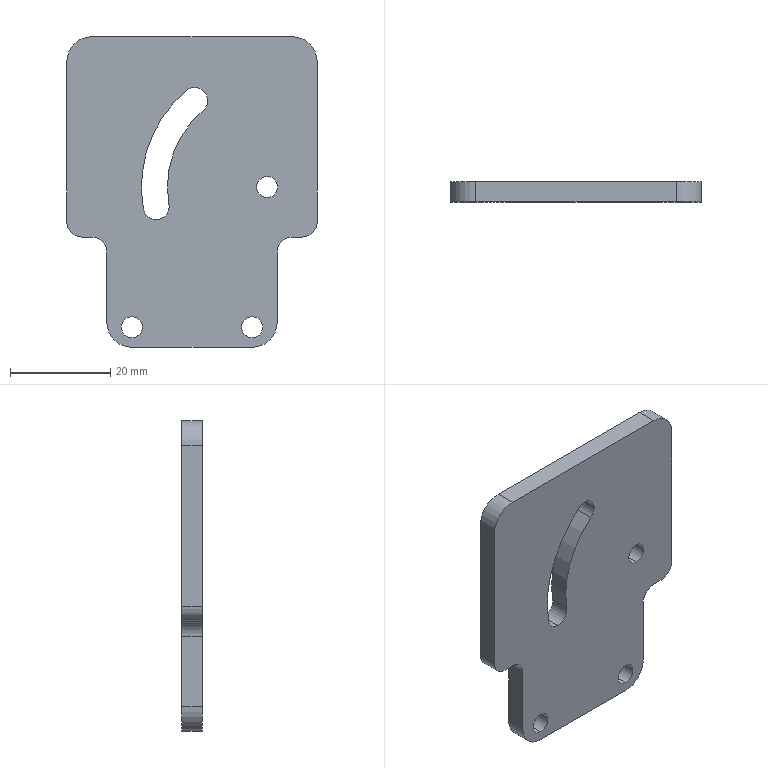Part | SolidWorks | features BaseBody 1 | 1 solid | 29 faces | box 50 x 4 x 62 mm | volume 10165 mm3 | cylinder 19 | plane 10 | commonest cylinder face diameters 4.2 x6 6 x4 10 x4 5.2 x3 39.8 x1 50.2 x1
STEP:
#1=CARTESIAN_POINT('',(-27.,0.,-25.9));
#2=VERTEX_POINT('',#1);
#3=CARTESIAN_POINT('',(-27.,0.,-30.1));
#4=VERTEX_POINT('',#3);
#5=CARTESIAN_POINT('',(-27.,0.,-28.));
#6=DIRECTION('',(0.,-1.,0.));
#7=DIRECTION('',(0.,0.,1.));
#8=AXIS2_PLACEMENT_3D('',#5,#6,#7);
#9=CIRCLE('',#8,2.1);
#10=EDGE_CURVE('',#2,#4,#9,.T.);
#11=ORIENTED_EDGE('',*,*,#10,.T.);
#12=CARTESIAN_POINT('',(-27.,4.,-30.1));
#13=VERTEX_POINT('',#12);
#14=CARTESIAN_POINT('',(-27.,0.,-30.1));
#15=DIRECTION('',(0.,1.,0.));
#16=VECTOR('',#15,1000.);
#17=LINE('',#14,#16);
#18=EDGE_CURVE('',#4,#13,#17,.T.);
#19=ORIENTED_EDGE('',*,*,#18,.T.);
#20=CARTESIAN_POINT('',(-27.,4.,-25.9));
#21=VERTEX_POINT('',#20);
#22=CARTESIAN_POINT('',(-27.,4.,-28.));
#23=DIRECTION('',(0.,-1.,0.));
#24=DIRECTION('',(0.,0.,1.));
#25=AXIS2_PLACEMENT_3D('',#22,#23,#24);
#26=CIRCLE('',#25,2.1);
#27=EDGE_CURVE('',#21,#13,#26,.T.);
#28=ORIENTED_EDGE('',*,*,#27,.F.);
#29=CARTESIAN_POINT('',(-27.,0.,-25.9));
#30=DIRECTION('',(0.,1.,0.));
#31=VECTOR('',#30,1000.);
#32=LINE('',#29,#31);
#33=EDGE_CURVE('',#2,#21,#32,.T.);
#34=ORIENTED_EDGE('',*,*,#33,.F.);
#35=EDGE_LOOP('',(#11,#19,#28,#34));
#36=FACE_OUTER_BOUND('',#35,.T.);
#37=CARTESIAN_POINT('',(-27.,0.,-28.));
#38=DIRECTION('',(0.,1.,0.));
#39=DIRECTION('',(0.,0.,1.));
#40=AXIS2_PLACEMENT_3D('',#37,#38,#39);
#41=CYLINDRICAL_SURFACE('',#40,2.1);
#42=ADVANCED_FACE('',(#36),#41,.F.);
#43=CARTESIAN_POINT('',(-3.,0.,-25.9));
#44=VERTEX_POINT('',#43);
#45=CARTESIAN_POINT('',(-3.,0.,-30.1));
#46=VERTEX_POINT('',#45);
#47=CARTESIAN_POINT('',(-3.,0.,-28.));
#48=DIRECTION('',(0.,-1.,0.));
#49=DIRECTION('',(0.,0.,1.));
#50=AXIS2_PLACEMENT_3D('',#47,#48,#49);
#51=CIRCLE('',#50,2.1);
#52=EDGE_CURVE('',#44,#46,#51,.T.);
#53=ORIENTED_EDGE('',*,*,#52,.T.);
#54=CARTESIAN_POINT('',(-3.,4.,-30.1));
#55=VERTEX_POINT('',#54);
#56=CARTESIAN_POINT('',(-3.,0.,-30.1));
#57=DIRECTION('',(0.,1.,0.));
#58=VECTOR('',#57,1000.);
#59=LINE('',#56,#58);
#60=EDGE_CURVE('',#46,#55,#59,.T.);
#61=ORIENTED_EDGE('',*,*,#60,.T.);
#62=CARTESIAN_POINT('',(-3.,4.,-25.9));
#63=VERTEX_POINT('',#62);
#64=CARTESIAN_POINT('',(-3.,4.,-28.));
#65=DIRECTION('',(0.,-1.,0.));
#66=DIRECTION('',(0.,0.,1.));
#67=AXIS2_PLACEMENT_3D('',#64,#65,#66);
#68=CIRCLE('',#67,2.1);
#69=EDGE_CURVE('',#63,#55,#68,.T.);
#70=ORIENTED_EDGE('',*,*,#69,.F.);
#71=CARTESIAN_POINT('',(-3.,0.,-25.9));
#72=DIRECTION('',(0.,1.,0.));
#73=VECTOR('',#72,1000.);
#74=LINE('',#71,#73);
#75=EDGE_CURVE('',#44,#63,#74,.T.);
#76=ORIENTED_EDGE('',*,*,#75,.F.);
#77=EDGE_LOOP('',(#53,#61,#70,#76));
#78=FACE_OUTER_BOUND('',#77,.T.);
#79=CARTESIAN_POINT('',(-3.,0.,-28.));
#80=DIRECTION('',(0.,1.,0.));
#81=DIRECTION('',(0.,0.,1.));
#82=AXIS2_PLACEMENT_3D('',#79,#80,#81);
#83=CYLINDRICAL_SURFACE('',#82,2.1);
#84=ADVANCED_FACE('',(#78),#83,.F.);
#85=CARTESIAN_POINT('',(-22.158,4.,-6.507));
#86=VERTEX_POINT('',#85);
#87=CARTESIAN_POINT('',(-19.598,4.,-3.456));
#88=VERTEX_POINT('',#87);
#89=CARTESIAN_POINT('',(-22.158,4.,-3.907));
#90=DIRECTION('',(0.,-1.,0.));
#91=DIRECTION('',(0.,0.,-1.));
#92=AXIS2_PLACEMENT_3D('',#89,#90,#91);
#93=CIRCLE('',#92,2.6);
#94=EDGE_CURVE('',#86,#88,#93,.T.);
#95=ORIENTED_EDGE('',*,*,#94,.F.);
#96=CARTESIAN_POINT('',(-22.158,0.,-6.507));
#97=VERTEX_POINT('',#96);
#98=CARTESIAN_POINT('',(-22.158,4.,-6.507));
#99=DIRECTION('',(0.,-1.,0.));
#100=VECTOR('',#99,1000.);
#101=LINE('',#98,#100);
#102=EDGE_CURVE('',#86,#97,#101,.T.);
#103=ORIENTED_EDGE('',*,*,#102,.T.);
#104=CARTESIAN_POINT('',(-19.598,0.,-3.456));
#105=VERTEX_POINT('',#104);
#106=CARTESIAN_POINT('',(-22.158,0.,-3.907));
#107=DIRECTION('',(0.,-1.,0.));
#108=DIRECTION('',(0.,0.,-1.));
#109=AXIS2_PLACEMENT_3D('',#106,#107,#108);
#110=CIRCLE('',#109,2.6);
#111=EDGE_CURVE('',#97,#105,#110,.T.);
#112=ORIENTED_EDGE('',*,*,#111,.T.);
#113=CARTESIAN_POINT('',(-19.598,4.,-3.456));
#114=DIRECTION('',(0.,-1.,0.));
#115=VECTOR('',#114,1000.);
#116=LINE('',#113,#115);
#117=EDGE_CURVE('',#88,#105,#116,.T.);
#118=ORIENTED_EDGE('',*,*,#117,.F.);
#119=EDGE_LOOP('',(#95,#103,#112,#118));
#120=FACE_OUTER_BOUND('',#119,.T.);
#121=CARTESIAN_POINT('',(-22.158,4.,-3.907));
#122=DIRECTION('',(0.,-1.,0.));
#123=DIRECTION('',(0.,0.,-1.));
#124=AXIS2_PLACEMENT_3D('',#121,#122,#123);
#125=CYLINDRICAL_SURFACE('',#124,2.6);
#126=ADVANCED_FACE('',(#120),#125,.F.);
#127=CARTESIAN_POINT('',(0.,4.,2.1));
#128=VERTEX_POINT('',#127);
#129=CARTESIAN_POINT('',(0.,4.,-2.1));
#130=VERTEX_POINT('',#129);
#131=CARTESIAN_POINT('',(0.,4.,0.));
#132=DIRECTION('',(0.,-1.,0.));
#133=DIRECTION('',(0.,0.,-1.));
#134=AXIS2_PLACEMENT_3D('',#131,#132,#133);
#135=CIRCLE('',#134,2.1);
#136=EDGE_CURVE('',#128,#130,#135,.T.);
#137=ORIENTED_EDGE('',*,*,#136,.F.);
#138=CARTESIAN_POINT('',(0.,0.,2.1));
#139=VERTEX_POINT('',#138);
#140=CARTESIAN_POINT('',(0.,4.,2.1));
#141=DIRECTION('',(0.,-1.,0.));
#142=VECTOR('',#141,1000.);
#143=LINE('',#140,#142);
#144=EDGE_CURVE('',#128,#139,#143,.T.);
#145=ORIENTED_EDGE('',*,*,#144,.T.);
#146=CARTESIAN_POINT('',(0.,0.,-2.1));
#147=VERTEX_POINT('',#146);
#148=CARTESIAN_POINT('',(0.,0.,0.));
#149=DIRECTION('',(0.,-1.,0.));
#150=DIRECTION('',(0.,0.,-1.));
#151=AXIS2_PLACEMENT_3D('',#148,#149,#150);
#152=CIRCLE('',#151,2.1);
#153=EDGE_CURVE('',#139,#147,#152,.T.);
#154=ORIENTED_EDGE('',*,*,#153,.T.);
#155=CARTESIAN_POINT('',(0.,4.,-2.1));
#156=DIRECTION('',(0.,-1.,0.));
#157=VECTOR('',#156,1000.);
#158=LINE('',#155,#157);
#159=EDGE_CURVE('',#130,#147,#158,.T.);
#160=ORIENTED_EDGE('',*,*,#159,.F.);
#161=EDGE_LOOP('',(#137,#145,#154,#160));
#162=FACE_OUTER_BOUND('',#161,.T.);
#163=CARTESIAN_POINT('',(0.,4.,0.));
#164=DIRECTION('',(0.,-1.,0.));
#165=DIRECTION('',(0.,0.,-1.));
#166=AXIS2_PLACEMENT_3D('',#163,#164,#165);
#167=CYLINDRICAL_SURFACE('',#166,2.1);
#168=ADVANCED_FACE('',(#162),#167,.F.);
#169=ORIENTED_EDGE('',*,*,#10,.F.);
#170=CARTESIAN_POINT('',(-27.,0.,-28.));
#171=DIRECTION('',(0.,-1.,0.));
#172=DIRECTION('',(0.,0.,1.));
#173=AXIS2_PLACEMENT_3D('',#170,#171,#172);
#174=CIRCLE('',#173,2.1);
#175=EDGE_CURVE('',#4,#2,#174,.T.);
#176=ORIENTED_EDGE('',*,*,#175,.F.);
#177=EDGE_LOOP('',(#169,#176));
#178=FACE_BOUND('',#177,.T.);
#179=ORIENTED_EDGE('',*,*,#52,.F.);
#180=CARTESIAN_POINT('',(-3.,0.,-28.));
#181=DIRECTION('',(0.,-1.,0.));
#182=DIRECTION('',(0.,0.,1.));
#183=AXIS2_PLACEMENT_3D('',#180,#181,#182);
#184=CIRCLE('',#183,2.1);
#185=EDGE_CURVE('',#46,#44,#184,.T.);
#186=ORIENTED_EDGE('',*,*,#185,.F.);
#187=EDGE_LOOP('',(#179,#186));
#188=FACE_BOUND('',#187,.T.);
#189=CARTESIAN_POINT('',(-24.719,0.,-4.359));
#190=VERTEX_POINT('',#189);
#191=CARTESIAN_POINT('',(-22.158,0.,-3.907));
#192=DIRECTION('',(0.,-1.,0.));
#193=DIRECTION('',(0.,0.,-1.));
#194=AXIS2_PLACEMENT_3D('',#191,#192,#193);
#195=CIRCLE('',#194,2.6);
#196=EDGE_CURVE('',#190,#97,#195,.T.);
#197=ORIENTED_EDGE('',*,*,#196,.F.);
#198=CARTESIAN_POINT('',(-16.134,0.,19.228));
#199=VERTEX_POINT('',#198);
#200=CARTESIAN_POINT('',(0.,0.,0.));
#201=DIRECTION('',(0.,-1.,0.));
#202=DIRECTION('',(0.,0.,-1.));
#203=AXIS2_PLACEMENT_3D('',#200,#201,#202);
#204=CIRCLE('',#203,25.1);
#205=EDGE_CURVE('',#199,#190,#204,.T.);
#206=ORIENTED_EDGE('',*,*,#205,.F.);
#207=CARTESIAN_POINT('',(-12.791,0.,15.244));
#208=VERTEX_POINT('',#207);
#209=CARTESIAN_POINT('',(-14.463,0.,17.236));
#210=DIRECTION('',(0.,-1.,0.));
#211=DIRECTION('',(0.,0.,-1.));
#212=AXIS2_PLACEMENT_3D('',#209,#210,#211);
#213=CIRCLE('',#212,2.6);
#214=EDGE_CURVE('',#208,#199,#213,.T.);
#215=ORIENTED_EDGE('',*,*,#214,.F.);
#216=CARTESIAN_POINT('',(0.,0.,0.));
#217=DIRECTION('',(0.,1.,0.));
#218=DIRECTION('',(0.,0.,-1.));
#219=AXIS2_PLACEMENT_3D('',#216,#217,#218);
#220=CIRCLE('',#219,19.9);
#221=EDGE_CURVE('',#105,#208,#220,.T.);
#222=ORIENTED_EDGE('',*,*,#221,.F.);
#223=ORIENTED_EDGE('',*,*,#111,.F.);
#224=EDGE_LOOP('',(#197,#206,#215,#222,#223));
#225=FACE_BOUND('',#224,.T.);
#226=CARTESIAN_POINT('',(2.,0.,-27.));
#227=VERTEX_POINT('',#226);
#228=CARTESIAN_POINT('',(-3.,0.,-32.));
#229=VERTEX_POINT('',#228);
#230=CARTESIAN_POINT('',(-3.,0.,-27.));
#231=DIRECTION('',(0.,1.,0.));
#232=DIRECTION('',(0.,0.,1.));
#233=AXIS2_PLACEMENT_3D('',#230,#231,#232);
#234=CIRCLE('',#233,5.);
#235=EDGE_CURVE('',#227,#229,#234,.T.);
#236=ORIENTED_EDGE('',*,*,#235,.F.);
#237=CARTESIAN_POINT('',(2.,0.,-13.));
#238=VERTEX_POINT('',#237);
#239=CARTESIAN_POINT('',(2.,0.,0.));
#240=DIRECTION('',(0.,0.,-1.));
#241=VECTOR('',#240,1000.);
#242=LINE('',#239,#241);
#243=EDGE_CURVE('',#238,#227,#242,.T.);
#244=ORIENTED_EDGE('',*,*,#243,.F.);
#245=CARTESIAN_POINT('',(5.,0.,-10.));
#246=VERTEX_POINT('',#245);
#247=CARTESIAN_POINT('',(5.,0.,-13.));
#248=DIRECTION('',(0.,-1.,0.));
#249=DIRECTION('',(0.,0.,-1.));
#250=AXIS2_PLACEMENT_3D('',#247,#248,#249);
#251=CIRCLE('',#250,3.);
#252=EDGE_CURVE('',#246,#238,#251,.T.);
#253=ORIENTED_EDGE('',*,*,#252,.F.);
#254=CARTESIAN_POINT('',(7.,0.,-10.));
#255=VERTEX_POINT('',#254);
#256=CARTESIAN_POINT('',(0.,0.,-10.));
#257=DIRECTION('',(-1.,0.,0.));
#258=VECTOR('',#257,1000.);
#259=LINE('',#256,#258);
#260=EDGE_CURVE('',#255,#246,#259,.T.);
#261=ORIENTED_EDGE('',*,*,#260,.F.);
#262=CARTESIAN_POINT('',(10.,0.,-7.));
#263=VERTEX_POINT('',#262);
#264=CARTESIAN_POINT('',(7.,0.,-7.));
#265=DIRECTION('',(0.,1.,0.));
#266=DIRECTION('',(0.,0.,-1.));
#267=AXIS2_PLACEMENT_3D('',#264,#265,#266);
#268=CIRCLE('',#267,3.);
#269=EDGE_CURVE('',#263,#255,#268,.T.);
#270=ORIENTED_EDGE('',*,*,#269,.F.);
#271=CARTESIAN_POINT('',(10.,0.,25.));
#272=VERTEX_POINT('',#271);
#273=CARTESIAN_POINT('',(10.,0.,0.));
#274=DIRECTION('',(0.,0.,-1.));
#275=VECTOR('',#274,1000.);
#276=LINE('',#273,#275);
#277=EDGE_CURVE('',#272,#263,#276,.T.);
#278=ORIENTED_EDGE('',*,*,#277,.F.);
#279=CARTESIAN_POINT('',(5.,0.,30.));
#280=VERTEX_POINT('',#279);
#281=CARTESIAN_POINT('',(5.,0.,25.));
#282=DIRECTION('',(0.,1.,0.));
#283=DIRECTION('',(0.,0.,-1.));
#284=AXIS2_PLACEMENT_3D('',#281,#282,#283);
#285=CIRCLE('',#284,5.);
#286=EDGE_CURVE('',#280,#272,#285,.T.);
#287=ORIENTED_EDGE('',*,*,#286,.F.);
#288=CARTESIAN_POINT('',(-35.,0.,30.));
#289=VERTEX_POINT('',#288);
#290=CARTESIAN_POINT('',(0.,0.,30.));
#291=DIRECTION('',(1.,0.,0.));
#292=VECTOR('',#291,1000.);
#293=LINE('',#290,#292);
#294=EDGE_CURVE('',#289,#280,#293,.T.);
#295=ORIENTED_EDGE('',*,*,#294,.F.);
#296=CARTESIAN_POINT('',(-40.,0.,25.));
#297=VERTEX_POINT('',#296);
#298=CARTESIAN_POINT('',(-35.,0.,25.));
#299=DIRECTION('',(0.,1.,0.));
#300=DIRECTION('',(0.,0.,-1.));
#301=AXIS2_PLACEMENT_3D('',#298,#299,#300);
#302=CIRCLE('',#301,5.);
#303=EDGE_CURVE('',#297,#289,#302,.T.);
#304=ORIENTED_EDGE('',*,*,#303,.F.);
#305=CARTESIAN_POINT('',(-40.,0.,-7.));
#306=VERTEX_POINT('',#305);
#307=CARTESIAN_POINT('',(-40.,0.,0.));
#308=DIRECTION('',(0.,0.,1.));
#309=VECTOR('',#308,1000.);
#310=LINE('',#307,#309);
#311=EDGE_CURVE('',#306,#297,#310,.T.);
#312=ORIENTED_EDGE('',*,*,#311,.F.);
#313=CARTESIAN_POINT('',(-37.,0.,-10.));
#314=VERTEX_POINT('',#313);
#315=CARTESIAN_POINT('',(-37.,0.,-7.));
#316=DIRECTION('',(0.,1.,0.));
#317=DIRECTION('',(0.,0.,-1.));
#318=AXIS2_PLACEMENT_3D('',#315,#316,#317);
#319=CIRCLE('',#318,3.);
#320=EDGE_CURVE('',#314,#306,#319,.T.);
#321=ORIENTED_EDGE('',*,*,#320,.F.);
#322=CARTESIAN_POINT('',(-35.,0.,-10.));
#323=VERTEX_POINT('',#322);
#324=CARTESIAN_POINT('',(0.,0.,-10.));
#325=DIRECTION('',(-1.,0.,0.));
#326=VECTOR('',#325,1000.);
#327=LINE('',#324,#326);
#328=EDGE_CURVE('',#323,#314,#327,.T.);
#329=ORIENTED_EDGE('',*,*,#328,.F.);
#330=CARTESIAN_POINT('',(-32.,0.,-13.));
#331=VERTEX_POINT('',#330);
#332=CARTESIAN_POINT('',(-35.,0.,-13.));
#333=DIRECTION('',(0.,-1.,0.));
#334=DIRECTION('',(0.,0.,1.));
#335=AXIS2_PLACEMENT_3D('',#332,#333,#334);
#336=CIRCLE('',#335,3.);
#337=EDGE_CURVE('',#331,#323,#336,.T.);
#338=ORIENTED_EDGE('',*,*,#337,.F.);
#339=CARTESIAN_POINT('',(-32.,0.,-27.));
#340=VERTEX_POINT('',#339);
#341=CARTESIAN_POINT('',(-32.,0.,0.));
#342=DIRECTION('',(0.,0.,1.));
#343=VECTOR('',#342,1000.);
#344=LINE('',#341,#343);
#345=EDGE_CURVE('',#340,#331,#344,.T.);
#346=ORIENTED_EDGE('',*,*,#345,.F.);
#347=CARTESIAN_POINT('',(-27.,0.,-32.));
#348=VERTEX_POINT('',#347);
#349=CARTESIAN_POINT('',(-27.,0.,-27.));
#350=DIRECTION('',(0.,1.,0.));
#351=DIRECTION('',(0.,0.,-1.));
#352=AXIS2_PLACEMENT_3D('',#349,#350,#351);
#353=CIRCLE('',#352,5.);
#354=EDGE_CURVE('',#348,#340,#353,.T.);
#355=ORIENTED_EDGE('',*,*,#354,.F.);
#356=CARTESIAN_POINT('',(0.,0.,-32.));
#357=DIRECTION('',(-1.,0.,0.));
#358=VECTOR('',#357,1000.);
#359=LINE('',#356,#358);
#360=EDGE_CURVE('',#229,#348,#359,.T.);
#361=ORIENTED_EDGE('',*,*,#360,.F.);
#362=EDGE_LOOP('',(#236,#244,#253,#261,#270,#278,#287,#295,#304,#312,#321,#329,#338,#346,#355,#361));
#363=FACE_OUTER_BOUND('',#362,.T.);
#364=CARTESIAN_POINT('',(0.,0.,0.));
#365=DIRECTION('',(0.,-1.,0.));
#366=DIRECTION('',(0.,0.,-1.));
#367=AXIS2_PLACEMENT_3D('',#364,#365,#366);
#368=CIRCLE('',#367,2.1);
#369=EDGE_CURVE('',#147,#139,#368,.T.);
#370=ORIENTED_EDGE('',*,*,#369,.F.);
#371=ORIENTED_EDGE('',*,*,#153,.F.);
#372=EDGE_LOOP('',(#370,#371));
#373=FACE_BOUND('',#372,.T.);
#374=CARTESIAN_POINT('',(0.,0.,0.));
#375=DIRECTION('',(0.,1.,0.));
#376=DIRECTION('',(0.,0.,1.));
#377=AXIS2_PLACEMENT_3D('',#374,#375,#376);
#378=PLANE('',#377);
#379=ADVANCED_FACE('',(#178,#188,#225,#363,#373),#378,.F.);
#380=ORIENTED_EDGE('',*,*,#18,.F.);
#381=ORIENTED_EDGE('',*,*,#175,.T.);
#382=ORIENTED_EDGE('',*,*,#33,.T.);
#383=CARTESIAN_POINT('',(-27.,4.,-28.));
#384=DIRECTION('',(0.,-1.,0.));
#385=DIRECTION('',(0.,0.,1.));
#386=AXIS2_PLACEMENT_3D('',#383,#384,#385);
#387=CIRCLE('',#386,2.1);
#388=EDGE_CURVE('',#13,#21,#387,.T.);
#389=ORIENTED_EDGE('',*,*,#388,.F.);
#390=EDGE_LOOP('',(#380,#381,#382,#389));
#391=FACE_OUTER_BOUND('',#390,.T.);
#392=CARTESIAN_POINT('',(-27.,0.,-28.));
#393=DIRECTION('',(0.,1.,0.));
#394=DIRECTION('',(0.,0.,1.));
#395=AXIS2_PLACEMENT_3D('',#392,#393,#394);
#396=CYLINDRICAL_SURFACE('',#395,2.1);
#397=ADVANCED_FACE('',(#391),#396,.F.);
#398=ORIENTED_EDGE('',*,*,#60,.F.);
#399=ORIENTED_EDGE('',*,*,#185,.T.);
#400=ORIENTED_EDGE('',*,*,#75,.T.);
#401=CARTESIAN_POINT('',(-3.,4.,-28.));
#402=DIRECTION('',(0.,-1.,0.));
#403=DIRECTION('',(0.,0.,1.));
#404=AXIS2_PLACEMENT_3D('',#401,#402,#403);
#405=CIRCLE('',#404,2.1);
#406=EDGE_CURVE('',#55,#63,#405,.T.);
#407=ORIENTED_EDGE('',*,*,#406,.F.);
#408=EDGE_LOOP('',(#398,#399,#400,#407));
#409=FACE_OUTER_BOUND('',#408,.T.);
#410=CARTESIAN_POINT('',(-3.,0.,-28.));
#411=DIRECTION('',(0.,1.,0.));
#412=DIRECTION('',(0.,0.,1.));
#413=AXIS2_PLACEMENT_3D('',#410,#411,#412);
#414=CYLINDRICAL_SURFACE('',#413,2.1);
#415=ADVANCED_FACE('',(#409),#414,.F.);
#416=ORIENTED_EDGE('',*,*,#102,.F.);
#417=CARTESIAN_POINT('',(-24.719,4.,-4.359));
#418=VERTEX_POINT('',#417);
#419=CARTESIAN_POINT('',(-22.158,4.,-3.907));
#420=DIRECTION('',(0.,-1.,0.));
#421=DIRECTION('',(0.,0.,-1.));
#422=AXIS2_PLACEMENT_3D('',#419,#420,#421);
#423=CIRCLE('',#422,2.6);
#424=EDGE_CURVE('',#418,#86,#423,.T.);
#425=ORIENTED_EDGE('',*,*,#424,.F.);
#426=CARTESIAN_POINT('',(-24.719,4.,-4.359));
#427=DIRECTION('',(0.,1.,0.));
#428=VECTOR('',#427,1000.);
#429=LINE('',#426,#428);
#430=EDGE_CURVE('',#190,#418,#429,.T.);
#431=ORIENTED_EDGE('',*,*,#430,.F.);
#432=ORIENTED_EDGE('',*,*,#196,.T.);
#433=EDGE_LOOP('',(#416,#425,#431,#432));
#434=FACE_OUTER_BOUND('',#433,.T.);
#435=CARTESIAN_POINT('',(-22.158,4.,-3.907));
#436=DIRECTION('',(0.,-1.,0.));
#437=DIRECTION('',(0.,0.,-1.));
#438=AXIS2_PLACEMENT_3D('',#435,#436,#437);
#439=CYLINDRICAL_SURFACE('',#438,2.6);
#440=ADVANCED_FACE('',(#434),#439,.F.);
#441=ORIENTED_EDGE('',*,*,#430,.T.);
#442=CARTESIAN_POINT('',(-16.134,4.,19.228));
#443=VERTEX_POINT('',#442);
#444=CARTESIAN_POINT('',(0.,4.,0.));
#445=DIRECTION('',(0.,-1.,0.));
#446=DIRECTION('',(0.,0.,-1.));
#447=AXIS2_PLACEMENT_3D('',#444,#445,#446);
#448=CIRCLE('',#447,25.1);
#449=EDGE_CURVE('',#443,#418,#448,.T.);
#450=ORIENTED_EDGE('',*,*,#449,.F.);
#451=CARTESIAN_POINT('',(-16.134,4.,19.228));
#452=DIRECTION('',(0.,1.,0.));
#453=VECTOR('',#452,1000.);
#454=LINE('',#451,#453);
#455=EDGE_CURVE('',#199,#443,#454,.T.);
#456=ORIENTED_EDGE('',*,*,#455,.F.);
#457=ORIENTED_EDGE('',*,*,#205,.T.);
#458=EDGE_LOOP('',(#441,#450,#456,#457));
#459=FACE_OUTER_BOUND('',#458,.T.);
#460=CARTESIAN_POINT('',(0.,4.,0.));
#461=DIRECTION('',(0.,-1.,0.));
#462=DIRECTION('',(0.,0.,-1.));
#463=AXIS2_PLACEMENT_3D('',#460,#461,#462);
#464=CYLINDRICAL_SURFACE('',#463,25.1);
#465=ADVANCED_FACE('',(#459),#464,.F.);
#466=ORIENTED_EDGE('',*,*,#455,.T.);
#467=CARTESIAN_POINT('',(-12.791,4.,15.244));
#468=VERTEX_POINT('',#467);
#469=CARTESIAN_POINT('',(-14.463,4.,17.236));
#470=DIRECTION('',(0.,-1.,0.));
#471=DIRECTION('',(0.,0.,-1.));
#472=AXIS2_PLACEMENT_3D('',#469,#470,#471);
#473=CIRCLE('',#472,2.6);
#474=EDGE_CURVE('',#468,#443,#473,.T.);
#475=ORIENTED_EDGE('',*,*,#474,.F.);
#476=CARTESIAN_POINT('',(-12.791,4.,15.244));
#477=DIRECTION('',(0.,1.,0.));
#478=VECTOR('',#477,1000.);
#479=LINE('',#476,#478);
#480=EDGE_CURVE('',#208,#468,#479,.T.);
#481=ORIENTED_EDGE('',*,*,#480,.F.);
#482=ORIENTED_EDGE('',*,*,#214,.T.);
#483=EDGE_LOOP('',(#466,#475,#481,#482));
#484=FACE_OUTER_BOUND('',#483,.T.);
#485=CARTESIAN_POINT('',(-14.463,4.,17.236));
#486=DIRECTION('',(0.,-1.,0.));
#487=DIRECTION('',(0.,0.,-1.));
#488=AXIS2_PLACEMENT_3D('',#485,#486,#487);
#489=CYLINDRICAL_SURFACE('',#488,2.6);
#490=ADVANCED_FACE('',(#484),#489,.F.);
#491=CARTESIAN_POINT('',(0.,4.,0.));
#492=DIRECTION('',(0.,-1.,0.));
#493=DIRECTION('',(0.,0.,-1.));
#494=AXIS2_PLACEMENT_3D('',#491,#492,#493);
#495=CIRCLE('',#494,19.9);
#496=EDGE_CURVE('',#468,#88,#495,.T.);
#497=ORIENTED_EDGE('',*,*,#496,.T.);
#498=ORIENTED_EDGE('',*,*,#117,.T.);
#499=ORIENTED_EDGE('',*,*,#221,.T.);
#500=ORIENTED_EDGE('',*,*,#480,.T.);
#501=EDGE_LOOP('',(#497,#498,#499,#500));
#502=FACE_OUTER_BOUND('',#501,.T.);
#503=CARTESIAN_POINT('',(0.,4.,0.));
#504=DIRECTION('',(0.,-1.,0.));
#505=DIRECTION('',(0.,0.,-1.));
#506=AXIS2_PLACEMENT_3D('',#503,#504,#505);
#507=CYLINDRICAL_SURFACE('',#506,19.9);
#508=ADVANCED_FACE('',(#502),#507,.T.);
#509=CARTESIAN_POINT('',(-3.,4.,-32.));
#510=VERTEX_POINT('',#509);
#511=CARTESIAN_POINT('',(-3.,0.,-32.));
#512=DIRECTION('',(0.,1.,0.));
#513=VECTOR('',#512,1000.);
#514=LINE('',#511,#513);
#515=EDGE_CURVE('',#229,#510,#514,.T.);
#516=ORIENTED_EDGE('',*,*,#515,.F.);
#517=ORIENTED_EDGE('',*,*,#360,.T.);
#518=CARTESIAN_POINT('',(-27.,4.,-32.));
#519=VERTEX_POINT('',#518);
#520=CARTESIAN_POINT('',(-27.,0.,-32.));
#521=DIRECTION('',(0.,-1.,0.));
#522=VECTOR('',#521,1000.);
#523=LINE('',#520,#522);
#524=EDGE_CURVE('',#519,#348,#523,.T.);
#525=ORIENTED_EDGE('',*,*,#524,.F.);
#526=CARTESIAN_POINT('',(0.,4.,-32.));
#527=DIRECTION('',(-1.,0.,0.));
#528=VECTOR('',#527,1000.);
#529=LINE('',#526,#528);
#530=EDGE_CURVE('',#510,#519,#529,.T.);
#531=ORIENTED_EDGE('',*,*,#530,.F.);
#532=EDGE_LOOP('',(#516,#517,#525,#531));
#533=FACE_OUTER_BOUND('',#532,.T.);
#534=CARTESIAN_POINT('',(0.,0.,-32.));
#535=DIRECTION('',(0.,0.,1.));
#536=DIRECTION('',(1.,0.,0.));
#537=AXIS2_PLACEMENT_3D('',#534,#535,#536);
#538=PLANE('',#537);
#539=ADVANCED_FACE('',(#533),#538,.F.);
#540=CARTESIAN_POINT('',(2.,4.,-27.));
#541=VERTEX_POINT('',#540);
#542=CARTESIAN_POINT('',(-3.,4.,-27.));
#543=DIRECTION('',(0.,-1.,0.));
#544=DIRECTION('',(0.,0.,1.));
#545=AXIS2_PLACEMENT_3D('',#542,#543,#544);
#546=CIRCLE('',#545,5.);
#547=EDGE_CURVE('',#510,#541,#546,.T.);
#548=ORIENTED_EDGE('',*,*,#547,.T.);
#549=CARTESIAN_POINT('',(2.,0.,-27.));
#550=DIRECTION('',(0.,-1.,0.));
#551=VECTOR('',#550,1000.);
#552=LINE('',#549,#551);
#553=EDGE_CURVE('',#541,#227,#552,.T.);
#554=ORIENTED_EDGE('',*,*,#553,.T.);
#555=ORIENTED_EDGE('',*,*,#235,.T.);
#556=ORIENTED_EDGE('',*,*,#515,.T.);
#557=EDGE_LOOP('',(#548,#554,#555,#556));
#558=FACE_OUTER_BOUND('',#557,.T.);
#559=CARTESIAN_POINT('',(-3.,0.,-27.));
#560=DIRECTION('',(0.,1.,0.));
#561=DIRECTION('',(0.,0.,1.));
#562=AXIS2_PLACEMENT_3D('',#559,#560,#561);
#563=CYLINDRICAL_SURFACE('',#562,5.);
#564=ADVANCED_FACE('',(#558),#563,.T.);
#565=ORIENTED_EDGE('',*,*,#553,.F.);
#566=CARTESIAN_POINT('',(2.,4.,-13.));
#567=VERTEX_POINT('',#566);
#568=CARTESIAN_POINT('',(2.,4.,0.));
#569=DIRECTION('',(0.,0.,-1.));
#570=VECTOR('',#569,1000.);
#571=LINE('',#568,#570);
#572=EDGE_CURVE('',#567,#541,#571,.T.);
#573=ORIENTED_EDGE('',*,*,#572,.F.);
#574=CARTESIAN_POINT('',(2.,0.,-13.));
#575=DIRECTION('',(0.,1.,0.));
#576=VECTOR('',#575,1000.);
#577=LINE('',#574,#576);
#578=EDGE_CURVE('',#238,#567,#577,.T.);
#579=ORIENTED_EDGE('',*,*,#578,.F.);
#580=ORIENTED_EDGE('',*,*,#243,.T.);
#581=EDGE_LOOP('',(#565,#573,#579,#580));
#582=FACE_OUTER_BOUND('',#581,.T.);
#583=CARTESIAN_POINT('',(2.,0.,0.));
#584=DIRECTION('',(-1.,0.,0.));
#585=DIRECTION('',(0.,0.,1.));
#586=AXIS2_PLACEMENT_3D('',#583,#584,#585);
#587=PLANE('',#586);
#588=ADVANCED_FACE('',(#582),#587,.F.);
#589=ORIENTED_EDGE('',*,*,#578,.T.);
#590=CARTESIAN_POINT('',(5.,4.,-10.));
#591=VERTEX_POINT('',#590);
#592=CARTESIAN_POINT('',(5.,4.,-13.));
#593=DIRECTION('',(0.,-1.,0.));
#594=DIRECTION('',(0.,0.,-1.));
#595=AXIS2_PLACEMENT_3D('',#592,#593,#594);
#596=CIRCLE('',#595,3.);
#597=EDGE_CURVE('',#591,#567,#596,.T.);
#598=ORIENTED_EDGE('',*,*,#597,.F.);
#599=CARTESIAN_POINT('',(5.,4.,-10.));
#600=DIRECTION('',(0.,1.,0.));
#601=VECTOR('',#600,1000.);
#602=LINE('',#599,#601);
#603=EDGE_CURVE('',#246,#591,#602,.T.);
#604=ORIENTED_EDGE('',*,*,#603,.F.);
#605=ORIENTED_EDGE('',*,*,#252,.T.);
#606=EDGE_LOOP('',(#589,#598,#604,#605));
#607=FACE_OUTER_BOUND('',#606,.T.);
#608=CARTESIAN_POINT('',(5.,4.,-13.));
#609=DIRECTION('',(0.,-1.,0.));
#610=DIRECTION('',(0.,0.,-1.));
#611=AXIS2_PLACEMENT_3D('',#608,#609,#610);
#612=CYLINDRICAL_SURFACE('',#611,3.);
#613=ADVANCED_FACE('',(#607),#612,.F.);
#614=CARTESIAN_POINT('',(7.,4.,-10.));
#615=VERTEX_POINT('',#614);
#616=CARTESIAN_POINT('',(7.,4.,-10.));
#617=DIRECTION('',(0.,1.,0.));
#618=VECTOR('',#617,1000.);
#619=LINE('',#616,#618);
#620=EDGE_CURVE('',#255,#615,#619,.T.);
#621=ORIENTED_EDGE('',*,*,#620,.F.);
#622=ORIENTED_EDGE('',*,*,#260,.T.);
#623=ORIENTED_EDGE('',*,*,#603,.T.);
#624=CARTESIAN_POINT('',(-40.,4.,-10.));
#625=DIRECTION('',(-1.,0.,0.));
#626=VECTOR('',#625,1000.);
#627=LINE('',#624,#626);
#628=EDGE_CURVE('',#615,#591,#627,.T.);
#629=ORIENTED_EDGE('',*,*,#628,.F.);
#630=EDGE_LOOP('',(#621,#622,#623,#629));
#631=FACE_OUTER_BOUND('',#630,.T.);
#632=CARTESIAN_POINT('',(-40.,4.,-10.));
#633=DIRECTION('',(0.,0.,1.));
#634=DIRECTION('',(1.,0.,0.));
#635=AXIS2_PLACEMENT_3D('',#632,#633,#634);
#636=PLANE('',#635);
#637=ADVANCED_FACE('',(#631),#636,.F.);
#638=ORIENTED_EDGE('',*,*,#269,.T.);
#639=ORIENTED_EDGE('',*,*,#620,.T.);
#640=CARTESIAN_POINT('',(10.,4.,-7.));
#641=VERTEX_POINT('',#640);
#642=CARTESIAN_POINT('',(7.,4.,-7.));
#643=DIRECTION('',(0.,-1.,0.));
#644=DIRECTION('',(0.,0.,-1.));
#645=AXIS2_PLACEMENT_3D('',#642,#643,#644);
#646=CIRCLE('',#645,3.);
#647=EDGE_CURVE('',#615,#641,#646,.T.);
#648=ORIENTED_EDGE('',*,*,#647,.T.);
#649=CARTESIAN_POINT('',(10.,4.,-7.));
#650=DIRECTION('',(0.,-1.,0.));
#651=VECTOR('',#650,1000.);
#652=LINE('',#649,#651);
#653=EDGE_CURVE('',#641,#263,#652,.T.);
#654=ORIENTED_EDGE('',*,*,#653,.T.);
#655=EDGE_LOOP('',(#638,#639,#648,#654));
#656=FACE_OUTER_BOUND('',#655,.T.);
#657=CARTESIAN_POINT('',(7.,4.,-7.));
#658=DIRECTION('',(0.,-1.,0.));
#659=DIRECTION('',(0.,0.,-1.));
#660=AXIS2_PLACEMENT_3D('',#657,#658,#659);
#661=CYLINDRICAL_SURFACE('',#660,3.);
#662=ADVANCED_FACE('',(#656),#661,.T.);
#663=CARTESIAN_POINT('',(10.,4.,25.));
#664=VERTEX_POINT('',#663);
#665=CARTESIAN_POINT('',(10.,4.,25.));
#666=DIRECTION('',(0.,1.,0.));
#667=VECTOR('',#666,1000.);
#668=LINE('',#665,#667);
#669=EDGE_CURVE('',#272,#664,#668,.T.);
#670=ORIENTED_EDGE('',*,*,#669,.F.);
#671=ORIENTED_EDGE('',*,*,#277,.T.);
#672=ORIENTED_EDGE('',*,*,#653,.F.);
#673=CARTESIAN_POINT('',(10.,4.,-10.));
#674=DIRECTION('',(0.,0.,-1.));
#675=VECTOR('',#674,1000.);
#676=LINE('',#673,#675);
#677=EDGE_CURVE('',#664,#641,#676,.T.);
#678=ORIENTED_EDGE('',*,*,#677,.F.);
#679=EDGE_LOOP('',(#670,#671,#672,#678));
#680=FACE_OUTER_BOUND('',#679,.T.);
#681=CARTESIAN_POINT('',(10.,4.,-10.));
#682=DIRECTION('',(-1.,0.,0.));
#683=DIRECTION('',(0.,0.,1.));
#684=AXIS2_PLACEMENT_3D('',#681,#682,#683);
#685=PLANE('',#684);
#686=ADVANCED_FACE('',(#680),#685,.F.);
#687=ORIENTED_EDGE('',*,*,#286,.T.);
#688=ORIENTED_EDGE('',*,*,#669,.T.);
#689=CARTESIAN_POINT('',(5.,4.,30.));
#690=VERTEX_POINT('',#689);
#691=CARTESIAN_POINT('',(5.,4.,25.));
#692=DIRECTION('',(0.,-1.,0.));
#693=DIRECTION('',(0.,0.,-1.));
#694=AXIS2_PLACEMENT_3D('',#691,#692,#693);
#695=CIRCLE('',#694,5.);
#696=EDGE_CURVE('',#664,#690,#695,.T.);
#697=ORIENTED_EDGE('',*,*,#696,.T.);
#698=CARTESIAN_POINT('',(5.,4.,30.));
#699=DIRECTION('',(0.,-1.,0.));
#700=VECTOR('',#699,1000.);
#701=LINE('',#698,#700);
#702=EDGE_CURVE('',#690,#280,#701,.T.);
#703=ORIENTED_EDGE('',*,*,#702,.T.);
#704=EDGE_LOOP('',(#687,#688,#697,#703));
#705=FACE_OUTER_BOUND('',#704,.T.);
#706=CARTESIAN_POINT('',(5.,4.,25.));
#707=DIRECTION('',(0.,-1.,0.));
#708=DIRECTION('',(0.,0.,-1.));
#709=AXIS2_PLACEMENT_3D('',#706,#707,#708);
#710=CYLINDRICAL_SURFACE('',#709,5.);
#711=ADVANCED_FACE('',(#705),#710,.T.);
#712=CARTESIAN_POINT('',(-35.,4.,30.));
#713=VERTEX_POINT('',#712);
#714=CARTESIAN_POINT('',(-35.,4.,30.));
#715=DIRECTION('',(0.,1.,0.));
#716=VECTOR('',#715,1000.);
#717=LINE('',#714,#716);
#718=EDGE_CURVE('',#289,#713,#717,.T.);
#719=ORIENTED_EDGE('',*,*,#718,.F.);
#720=ORIENTED_EDGE('',*,*,#294,.T.);
#721=ORIENTED_EDGE('',*,*,#702,.F.);
#722=CARTESIAN_POINT('',(-40.,4.,30.));
#723=DIRECTION('',(1.,0.,0.));
#724=VECTOR('',#723,1000.);
#725=LINE('',#722,#724);
#726=EDGE_CURVE('',#713,#690,#725,.T.);
#727=ORIENTED_EDGE('',*,*,#726,.F.);
#728=EDGE_LOOP('',(#719,#720,#721,#727));
#729=FACE_OUTER_BOUND('',#728,.T.);
#730=CARTESIAN_POINT('',(-40.,4.,30.));
#731=DIRECTION('',(0.,0.,-1.));
#732=DIRECTION('',(-1.,0.,0.));
#733=AXIS2_PLACEMENT_3D('',#730,#731,#732);
#734=PLANE('',#733);
#735=ADVANCED_FACE('',(#729),#734,.F.);
#736=ORIENTED_EDGE('',*,*,#303,.T.);
#737=ORIENTED_EDGE('',*,*,#718,.T.);
#738=CARTESIAN_POINT('',(-40.,4.,25.));
#739=VERTEX_POINT('',#738);
#740=CARTESIAN_POINT('',(-35.,4.,25.));
#741=DIRECTION('',(0.,-1.,0.));
#742=DIRECTION('',(0.,0.,-1.));
#743=AXIS2_PLACEMENT_3D('',#740,#741,#742);
#744=CIRCLE('',#743,5.);
#745=EDGE_CURVE('',#713,#739,#744,.T.);
#746=ORIENTED_EDGE('',*,*,#745,.T.);
#747=CARTESIAN_POINT('',(-40.,4.,25.));
#748=DIRECTION('',(0.,-1.,0.));
#749=VECTOR('',#748,1000.);
#750=LINE('',#747,#749);
#751=EDGE_CURVE('',#739,#297,#750,.T.);
#752=ORIENTED_EDGE('',*,*,#751,.T.);
#753=EDGE_LOOP('',(#736,#737,#746,#752));
#754=FACE_OUTER_BOUND('',#753,.T.);
#755=CARTESIAN_POINT('',(-35.,4.,25.));
#756=DIRECTION('',(0.,-1.,0.));
#757=DIRECTION('',(0.,0.,-1.));
#758=AXIS2_PLACEMENT_3D('',#755,#756,#757);
#759=CYLINDRICAL_SURFACE('',#758,5.);
#760=ADVANCED_FACE('',(#754),#759,.T.);
#761=ORIENTED_EDGE('',*,*,#751,.F.);
#762=CARTESIAN_POINT('',(-40.,4.,-7.));
#763=VERTEX_POINT('',#762);
#764=CARTESIAN_POINT('',(-40.,4.,-10.));
#765=DIRECTION('',(0.,0.,1.));
#766=VECTOR('',#765,1000.);
#767=LINE('',#764,#766);
#768=EDGE_CURVE('',#763,#739,#767,.T.);
#769=ORIENTED_EDGE('',*,*,#768,.F.);
#770=CARTESIAN_POINT('',(-40.,4.,-7.));
#771=DIRECTION('',(0.,1.,0.));
#772=VECTOR('',#771,1000.);
#773=LINE('',#770,#772);
#774=EDGE_CURVE('',#306,#763,#773,.T.);
#775=ORIENTED_EDGE('',*,*,#774,.F.);
#776=ORIENTED_EDGE('',*,*,#311,.T.);
#777=EDGE_LOOP('',(#761,#769,#775,#776));
#778=FACE_OUTER_BOUND('',#777,.T.);
#779=CARTESIAN_POINT('',(-40.,4.,-10.));
#780=DIRECTION('',(1.,0.,0.));
#781=DIRECTION('',(0.,0.,-1.));
#782=AXIS2_PLACEMENT_3D('',#779,#780,#781);
#783=PLANE('',#782);
#784=ADVANCED_FACE('',(#778),#783,.F.);
#785=ORIENTED_EDGE('',*,*,#320,.T.);
#786=ORIENTED_EDGE('',*,*,#774,.T.);
#787=CARTESIAN_POINT('',(-37.,4.,-10.));
#788=VERTEX_POINT('',#787);
#789=CARTESIAN_POINT('',(-37.,4.,-7.));
#790=DIRECTION('',(0.,-1.,0.));
#791=DIRECTION('',(0.,0.,-1.));
#792=AXIS2_PLACEMENT_3D('',#789,#790,#791);
#793=CIRCLE('',#792,3.);
#794=EDGE_CURVE('',#763,#788,#793,.T.);
#795=ORIENTED_EDGE('',*,*,#794,.T.);
#796=CARTESIAN_POINT('',(-37.,4.,-10.));
#797=DIRECTION('',(0.,-1.,0.));
#798=VECTOR('',#797,1000.);
#799=LINE('',#796,#798);
#800=EDGE_CURVE('',#788,#314,#799,.T.);
#801=ORIENTED_EDGE('',*,*,#800,.T.);
#802=EDGE_LOOP('',(#785,#786,#795,#801));
#803=FACE_OUTER_BOUND('',#802,.T.);
#804=CARTESIAN_POINT('',(-37.,4.,-7.));
#805=DIRECTION('',(0.,-1.,0.));
#806=DIRECTION('',(0.,0.,-1.));
#807=AXIS2_PLACEMENT_3D('',#804,#805,#806);
#808=CYLINDRICAL_SURFACE('',#807,3.);
#809=ADVANCED_FACE('',(#803),#808,.T.);
#810=ORIENTED_EDGE('',*,*,#800,.F.);
#811=CARTESIAN_POINT('',(-35.,4.,-10.));
#812=VERTEX_POINT('',#811);
#813=CARTESIAN_POINT('',(-40.,4.,-10.));
#814=DIRECTION('',(-1.,0.,0.));
#815=VECTOR('',#814,1000.);
#816=LINE('',#813,#815);
#817=EDGE_CURVE('',#812,#788,#816,.T.);
#818=ORIENTED_EDGE('',*,*,#817,.F.);
#819=CARTESIAN_POINT('',(-35.,4.,-10.));
#820=DIRECTION('',(0.,1.,0.));
#821=VECTOR('',#820,1000.);
#822=LINE('',#819,#821);
#823=EDGE_CURVE('',#323,#812,#822,.T.);
#824=ORIENTED_EDGE('',*,*,#823,.F.);
#825=ORIENTED_EDGE('',*,*,#328,.T.);
#826=EDGE_LOOP('',(#810,#818,#824,#825));
#827=FACE_OUTER_BOUND('',#826,.T.);
#828=CARTESIAN_POINT('',(-40.,4.,-10.));
#829=DIRECTION('',(0.,0.,1.));
#830=DIRECTION('',(1.,0.,0.));
#831=AXIS2_PLACEMENT_3D('',#828,#829,#830);
#832=PLANE('',#831);
#833=ADVANCED_FACE('',(#827),#832,.F.);
#834=ORIENTED_EDGE('',*,*,#823,.T.);
#835=CARTESIAN_POINT('',(-32.,4.,-13.));
#836=VERTEX_POINT('',#835);
#837=CARTESIAN_POINT('',(-35.,4.,-13.));
#838=DIRECTION('',(0.,-1.,0.));
#839=DIRECTION('',(0.,0.,1.));
#840=AXIS2_PLACEMENT_3D('',#837,#838,#839);
#841=CIRCLE('',#840,3.);
#842=EDGE_CURVE('',#836,#812,#841,.T.);
#843=ORIENTED_EDGE('',*,*,#842,.F.);
#844=CARTESIAN_POINT('',(-32.,0.,-13.));
#845=DIRECTION('',(0.,1.,0.));
#846=VECTOR('',#845,1000.);
#847=LINE('',#844,#846);
#848=EDGE_CURVE('',#331,#836,#847,.T.);
#849=ORIENTED_EDGE('',*,*,#848,.F.);
#850=ORIENTED_EDGE('',*,*,#337,.T.);
#851=EDGE_LOOP('',(#834,#843,#849,#850));
#852=FACE_OUTER_BOUND('',#851,.T.);
#853=CARTESIAN_POINT('',(-35.,0.,-13.));
#854=DIRECTION('',(0.,1.,0.));
#855=DIRECTION('',(0.,0.,1.));
#856=AXIS2_PLACEMENT_3D('',#853,#854,#855);
#857=CYLINDRICAL_SURFACE('',#856,3.);
#858=ADVANCED_FACE('',(#852),#857,.F.);
#859=ORIENTED_EDGE('',*,*,#345,.T.);
#860=ORIENTED_EDGE('',*,*,#848,.T.);
#861=CARTESIAN_POINT('',(-32.,4.,-27.));
#862=VERTEX_POINT('',#861);
#863=CARTESIAN_POINT('',(-32.,4.,0.));
#864=DIRECTION('',(0.,0.,-1.));
#865=VECTOR('',#864,1000.);
#866=LINE('',#863,#865);
#867=EDGE_CURVE('',#836,#862,#866,.T.);
#868=ORIENTED_EDGE('',*,*,#867,.T.);
#869=CARTESIAN_POINT('',(-32.,0.,-27.));
#870=DIRECTION('',(0.,-1.,0.));
#871=VECTOR('',#870,1000.);
#872=LINE('',#869,#871);
#873=EDGE_CURVE('',#862,#340,#872,.T.);
#874=ORIENTED_EDGE('',*,*,#873,.T.);
#875=EDGE_LOOP('',(#859,#860,#868,#874));
#876=FACE_OUTER_BOUND('',#875,.T.);
#877=CARTESIAN_POINT('',(-32.,0.,0.));
#878=DIRECTION('',(-1.,0.,0.));
#879=DIRECTION('',(0.,0.,1.));
#880=AXIS2_PLACEMENT_3D('',#877,#878,#879);
#881=PLANE('',#880);
#882=ADVANCED_FACE('',(#876),#881,.T.);
#883=CARTESIAN_POINT('',(-27.,4.,-27.));
#884=DIRECTION('',(0.,-1.,0.));
#885=DIRECTION('',(0.,0.,-1.));
#886=AXIS2_PLACEMENT_3D('',#883,#884,#885);
#887=CIRCLE('',#886,5.);
#888=EDGE_CURVE('',#862,#519,#887,.T.);
#889=ORIENTED_EDGE('',*,*,#888,.T.);
#890=ORIENTED_EDGE('',*,*,#524,.T.);
#891=ORIENTED_EDGE('',*,*,#354,.T.);
#892=ORIENTED_EDGE('',*,*,#873,.F.);
#893=EDGE_LOOP('',(#889,#890,#891,#892));
#894=FACE_OUTER_BOUND('',#893,.T.);
#895=CARTESIAN_POINT('',(-27.,0.,-27.));
#896=DIRECTION('',(0.,-1.,0.));
#897=DIRECTION('',(0.,0.,-1.));
#898=AXIS2_PLACEMENT_3D('',#895,#896,#897);
#899=CYLINDRICAL_SURFACE('',#898,5.);
#900=ADVANCED_FACE('',(#894),#899,.T.);
#901=ORIENTED_EDGE('',*,*,#144,.F.);
#902=CARTESIAN_POINT('',(0.,4.,0.));
#903=DIRECTION('',(0.,-1.,0.));
#904=DIRECTION('',(0.,0.,-1.));
#905=AXIS2_PLACEMENT_3D('',#902,#903,#904);
#906=CIRCLE('',#905,2.1);
#907=EDGE_CURVE('',#130,#128,#906,.T.);
#908=ORIENTED_EDGE('',*,*,#907,.F.);
#909=ORIENTED_EDGE('',*,*,#159,.T.);
#910=ORIENTED_EDGE('',*,*,#369,.T.);
#911=EDGE_LOOP('',(#901,#908,#909,#910));
#912=FACE_OUTER_BOUND('',#911,.T.);
#913=CARTESIAN_POINT('',(0.,4.,0.));
#914=DIRECTION('',(0.,-1.,0.));
#915=DIRECTION('',(0.,0.,-1.));
#916=AXIS2_PLACEMENT_3D('',#913,#914,#915);
#917=CYLINDRICAL_SURFACE('',#916,2.1);
#918=ADVANCED_FACE('',(#912),#917,.F.);
#919=ORIENTED_EDGE('',*,*,#27,.T.);
#920=ORIENTED_EDGE('',*,*,#388,.T.);
#921=EDGE_LOOP('',(#919,#920));
#922=FACE_BOUND('',#921,.T.);
#923=ORIENTED_EDGE('',*,*,#69,.T.);
#924=ORIENTED_EDGE('',*,*,#406,.T.);
#925=EDGE_LOOP('',(#923,#924));
#926=FACE_BOUND('',#925,.T.);
#927=ORIENTED_EDGE('',*,*,#496,.F.);
#928=ORIENTED_EDGE('',*,*,#474,.T.);
#929=ORIENTED_EDGE('',*,*,#449,.T.);
#930=ORIENTED_EDGE('',*,*,#424,.T.);
#931=ORIENTED_EDGE('',*,*,#94,.T.);
#932=EDGE_LOOP('',(#927,#928,#929,#930,#931));
#933=FACE_BOUND('',#932,.T.);
#934=ORIENTED_EDGE('',*,*,#907,.T.);
#935=ORIENTED_EDGE('',*,*,#136,.T.);
#936=EDGE_LOOP('',(#934,#935));
#937=FACE_BOUND('',#936,.T.);
#938=ORIENTED_EDGE('',*,*,#628,.T.);
#939=ORIENTED_EDGE('',*,*,#597,.T.);
#940=ORIENTED_EDGE('',*,*,#572,.T.);
#941=ORIENTED_EDGE('',*,*,#547,.F.);
#942=ORIENTED_EDGE('',*,*,#530,.T.);
#943=ORIENTED_EDGE('',*,*,#888,.F.);
#944=ORIENTED_EDGE('',*,*,#867,.F.);
#945=ORIENTED_EDGE('',*,*,#842,.T.);
#946=ORIENTED_EDGE('',*,*,#817,.T.);
#947=ORIENTED_EDGE('',*,*,#794,.F.);
#948=ORIENTED_EDGE('',*,*,#768,.T.);
#949=ORIENTED_EDGE('',*,*,#745,.F.);
#950=ORIENTED_EDGE('',*,*,#726,.T.);
#951=ORIENTED_EDGE('',*,*,#696,.F.);
#952=ORIENTED_EDGE('',*,*,#677,.T.);
#953=ORIENTED_EDGE('',*,*,#647,.F.);
#954=EDGE_LOOP('',(#938,#939,#940,#941,#942,#943,#944,#945,#946,#947,#948,#949,#950,#951,#952,#953));
#955=FACE_OUTER_BOUND('',#954,.T.);
#956=CARTESIAN_POINT('',(0.,4.,0.));
#957=DIRECTION('',(0.,1.,0.));
#958=DIRECTION('',(0.,0.,1.));
#959=AXIS2_PLACEMENT_3D('',#956,#957,#958);
#960=PLANE('',#959);
#961=ADVANCED_FACE('',(#922,#926,#933,#937,#955),#960,.T.);
#962=CLOSED_SHELL('',(#42,#84,#126,#168,#379,#397,#415,#440,#465,#490,#508,#539,#564,#588,#613,#637,#662,#686,#711,#735,#760,#784,#809,#833,#858,#882,#900,#918,#961));
#963=MANIFOLD_SOLID_BREP('',#962);
#964=CARTESIAN_POINT('',(0.,0.,0.));
#965=DIRECTION('',(0.,0.,1.));
#966=DIRECTION('',(1.,0.,0.));
#967=AXIS2_PLACEMENT_3D('',#964,#965,#966);
#968=(LENGTH_UNIT()NAMED_UNIT(*)SI_UNIT(.MILLI.,.METRE.));
#969=UNCERTAINTY_MEASURE_WITH_UNIT(LENGTH_MEASURE(0.00001),#968,'','');
#970=(NAMED_UNIT(*)PLANE_ANGLE_UNIT()SI_UNIT($,.RADIAN.));
#971=(NAMED_UNIT(*)SI_UNIT($,.STERADIAN.)SOLID_ANGLE_UNIT());
#972=(GEOMETRIC_REPRESENTATION_CONTEXT(3)GLOBAL_UNCERTAINTY_ASSIGNED_CONTEXT((#969))GLOBAL_UNIT_ASSIGNED_CONTEXT((#968,#970,#971))REPRESENTATION_CONTEXT('',''));
#973=ADVANCED_BREP_SHAPE_REPRESENTATION('',(#963,#967),#972);